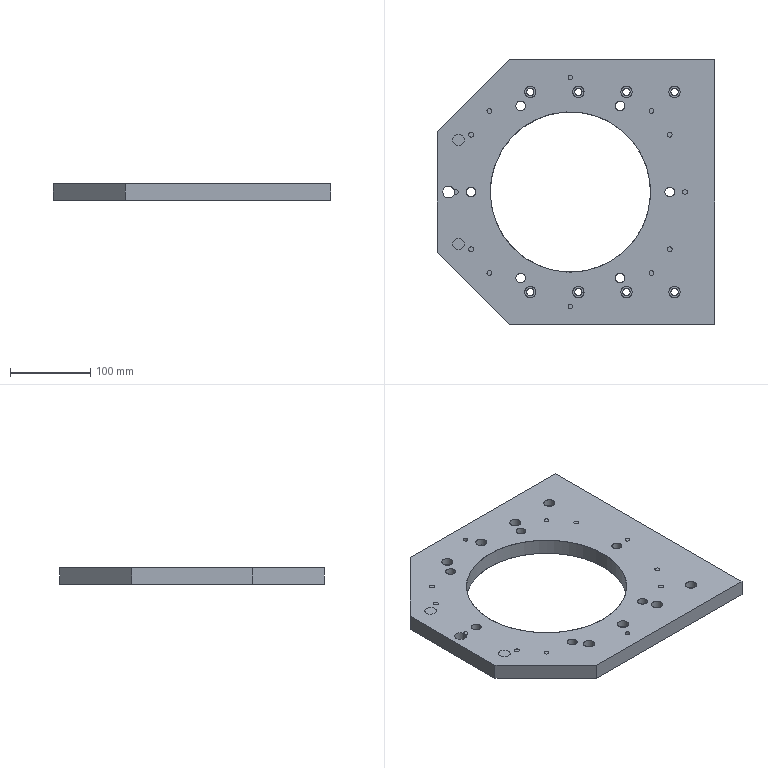NC program | NX | posted with a generic post | part box 346 x 330 x 20 mm
Lines 1 to 1039 of 2811:
N10 G17 G21 G94 G90
(ZLEVEL_PROFILE_COPY_1_1 , TOOL : D10)
N12 T10 M6
N14 G54
N16 G17 G0 G90 X174.775 Y181.218 S2200 M3
N18 G43 Z70. H10
N20 Z2.78
N22 G94 G1 Z-0.22 F2200.
N24 X170.649 Y178.835
N26 G3 X170.149 Y177.969 R1.
N28 G1 X170.15 Y173.041
N30 Y-83.
N32 G2 X168.642 Y-86.642 R5.15
N34 G1 X78.642 Y-176.642
N36 X74.993 Y-180.29
N38 G3 X74.734 Y-181.256 R1.
N40 G1 X75.955 Y-185.815
N42 Z2.78
N44 G0 Z2.56
N46 G1 Z-0.44
N48 X74.734 Y-181.256
N50 G2 X74.993 Y-180.29 R1.
N52 G1 X78.642 Y-176.642
N54 X168.642 Y-86.642
N56 G3 X170.15 Y-83. R5.15
N58 G1 Y173.041
N60 X170.149 Y177.969
N62 G2 X170.649 Y178.835 R1.
N64 G1 X174.775 Y181.218
N66 Z2.56
N68 G0 Z2.341
N70 G1 Z-0.659
N72 X170.649 Y178.835
N74 G3 X170.149 Y177.969 R1.
N76 G1 X170.15 Y173.041
N78 Y-83.
N80 G2 X168.642 Y-86.642 R5.15
N82 G1 X78.642 Y-176.642
N84 X74.993 Y-180.29
N86 G3 X74.734 Y-181.256 R1.
N88 G1 X75.955 Y-185.815
N90 Z2.341
N92 G0 Z2.121
N94 G1 Z-0.879
N96 X74.734 Y-181.256
N98 G2 X74.993 Y-180.29 R1.
N100 G1 X78.642 Y-176.642
N102 X168.642 Y-86.642
N104 G3 X170.15 Y-83. R5.15
N106 G1 Y173.041
N108 X170.149 Y177.969
N110 G2 X170.649 Y178.835 R1.
N112 G1 X174.775 Y181.218
N114 Z2.121
N116 G0 Z1.901
N118 G1 Z-1.099
N120 X170.649 Y178.835
N122 G3 X170.149 Y177.969 R1.
N124 G1 X170.15 Y173.041
N126 Y-83.
N128 G2 X168.642 Y-86.642 R5.15
N130 G1 X78.642 Y-176.642
N132 X74.993 Y-180.29
N134 G3 X74.734 Y-181.256 R1.
N136 G1 X75.955 Y-185.815
N138 Z1.901
N140 G0 Z1.681
N142 G1 Z-1.319
N144 X74.734 Y-181.256
N146 G2 X74.993 Y-180.29 R1.
N148 G1 X78.642 Y-176.642
N150 X168.642 Y-86.642
N152 G3 X170.15 Y-83. R5.15
N154 G1 Y173.041
N156 X170.149 Y177.969
N158 G2 X170.649 Y178.835 R1.
N160 G1 X174.775 Y181.218
N162 Z1.681
N164 G0 Z1.462
N166 G1 Z-1.538
N168 X170.649 Y178.835
N170 G3 X170.149 Y177.969 R1.
N172 G1 X170.15 Y173.041
N174 Y-83.
N176 G2 X168.642 Y-86.642 R5.15
N178 G1 X78.642 Y-176.642
N180 X74.993 Y-180.29
N182 G3 X74.734 Y-181.256 R1.
N184 G1 X75.955 Y-185.815
N186 Z1.462
N188 G0 Z1.242
N190 G1 Z-1.758
N192 X74.734 Y-181.256
N194 G2 X74.993 Y-180.29 R1.
N196 G1 X78.642 Y-176.642
N198 X168.642 Y-86.642
N200 G3 X170.15 Y-83. R5.15
N202 G1 Y173.041
N204 X170.149 Y177.969
N206 G2 X170.649 Y178.835 R1.
N208 G1 X174.775 Y181.218
N210 Z1.242
N212 G0 Z1.022
N214 G1 Z-1.978
N216 X170.649 Y178.835
N218 G3 X170.149 Y177.969 R1.
N220 G1 X170.15 Y173.041
N222 Y-83.
N224 G2 X168.642 Y-86.642 R5.15
N226 G1 X78.642 Y-176.642
N228 X74.993 Y-180.29
N230 G3 X74.734 Y-181.256 R1.
N232 G1 X75.955 Y-185.815
N234 Z1.022
N236 G0 Z0.802
N238 G1 Z-2.198
N240 X74.734 Y-181.256
N242 G2 X74.993 Y-180.29 R1.
N244 G1 X78.642 Y-176.642
N246 X168.642 Y-86.642
N248 G3 X170.15 Y-83. R5.15
N250 G1 Y173.041
N252 X170.149 Y177.969
N254 G2 X170.649 Y178.835 R1.
N256 G1 X174.775 Y181.218
N258 Z0.802
N260 G0 Z0.582
N262 G1 Z-2.418
N264 X170.649 Y178.835
N266 G3 X170.149 Y177.969 R1.
N268 G1 X170.15 Y173.041
N270 Y-83.
N272 G2 X168.642 Y-86.642 R5.15
N274 G1 X78.642 Y-176.642
N276 X74.993 Y-180.29
N278 G3 X74.734 Y-181.256 R1.
N280 G1 X75.955 Y-185.815
N282 Z0.582
N284 G0 Z0.363
N286 G1 Z-2.637
N288 X74.734 Y-181.256
N290 G2 X74.993 Y-180.29 R1.
N292 G1 X78.642 Y-176.642
N294 X168.642 Y-86.642
N296 G3 X170.15 Y-83. R5.15
N298 G1 Y173.041
N300 X170.149 Y177.969
N302 G2 X170.649 Y178.835 R1.
N304 G1 X174.775 Y181.218
N306 Z0.363
N308 G0 Z0.143
N310 G1 Z-2.857
N312 X170.649 Y178.835
N314 G3 X170.149 Y177.969 R1.
N316 G1 X170.15 Y173.041
N318 Y-83.
N320 G2 X168.642 Y-86.642 R5.15
N322 G1 X78.642 Y-176.642
N324 X74.993 Y-180.29
N326 G3 X74.734 Y-181.256 R1.
N328 G1 X75.955 Y-185.815
N330 Z0.143
N332 G0 Z-0.077
N334 G1 Z-3.077
N336 X74.734 Y-181.256
N338 G2 X74.993 Y-180.29 R1.
N340 G1 X78.642 Y-176.642
N342 X168.642 Y-86.642
N344 G3 X170.15 Y-83. R5.15
N346 G1 Y173.041
N348 X170.149 Y177.969
N350 G2 X170.649 Y178.835 R1.
N352 G1 X174.775 Y181.218
N354 Z-0.077
N356 G0 Z-0.297
N358 G1 Z-3.297
N360 X170.649 Y178.835
N362 G3 X170.149 Y177.969 R1.
N364 G1 X170.15 Y173.041
N366 Y-83.
N368 G2 X168.642 Y-86.642 R5.15
N370 G1 X78.642 Y-176.642
N372 X74.993 Y-180.29
N374 G3 X74.734 Y-181.256 R1.
N376 G1 X75.955 Y-185.815
N378 Z-0.297
N380 G0 Z-0.516
N382 G1 Z-3.516
N384 X74.734 Y-181.256
N386 G2 X74.993 Y-180.29 R1.
N388 G1 X78.642 Y-176.642
N390 X168.642 Y-86.642
N392 G3 X170.15 Y-83. R5.15
N394 G1 Y173.041
N396 X170.149 Y177.969
N398 G2 X170.649 Y178.835 R1.
N400 G1 X174.775 Y181.218
N402 Z-0.516
N404 G0 Z-0.736
N406 G1 Z-3.736
N408 X170.649 Y178.835
N410 G3 X170.149 Y177.969 R1.
N412 G1 X170.15 Y173.041
N414 Y-83.
N416 G2 X168.642 Y-86.642 R5.15
N418 G1 X78.642 Y-176.642
N420 X74.993 Y-180.29
N422 G3 X74.734 Y-181.256 R1.
N424 G1 X75.955 Y-185.815
N426 Z-0.736
N428 G0 Z-0.956
N430 G1 Z-3.956
N432 X74.734 Y-181.256
N434 G2 X74.993 Y-180.29 R1.
N436 G1 X78.642 Y-176.642
N438 X168.642 Y-86.642
N440 G3 X170.15 Y-83. R5.15
N442 G1 Y173.041
N444 X170.149 Y177.969
N446 G2 X170.649 Y178.835 R1.
N448 G1 X174.775 Y181.218
N450 Z-0.956
N452 G0 Z-1.176
N454 G1 Z-4.176
N456 X170.649 Y178.835
N458 G3 X170.149 Y177.969 R1.
N460 G1 X170.15 Y173.041
N462 Y-83.
N464 G2 X168.642 Y-86.642 R5.15
N466 G1 X78.642 Y-176.642
N468 X74.993 Y-180.29
N470 G3 X74.734 Y-181.256 R1.
N472 G1 X75.955 Y-185.815
N474 Z-1.176
N476 G0 Z-1.396
N478 G1 Z-4.396
N480 X74.734 Y-181.256
N482 G2 X74.993 Y-180.29 R1.
N484 G1 X78.642 Y-176.642
N486 X168.642 Y-86.642
N488 G3 X170.15 Y-83. R5.15
N490 G1 Y173.041
N492 X170.149 Y177.969
N494 G2 X170.649 Y178.835 R1.
N496 G1 X174.775 Y181.218
N498 Z-1.396
N500 G0 Z-1.615
N502 G1 Z-4.615
N504 X170.649 Y178.835
N506 G3 X170.149 Y177.969 R1.
N508 G1 X170.15 Y173.041
N510 Y-83.
N512 G2 X168.642 Y-86.642 R5.15
N514 G1 X78.642 Y-176.642
N516 X74.993 Y-180.29
N518 G3 X74.734 Y-181.256 R1.
N520 G1 X75.955 Y-185.815
N522 Z-1.615
N524 G0 Z-1.835
N526 G1 Z-4.835
N528 X74.734 Y-181.256
N530 G2 X74.993 Y-180.29 R1.
N532 G1 X78.642 Y-176.642
N534 X168.642 Y-86.642
N536 G3 X170.15 Y-83. R5.15
N538 G1 Y173.041
N540 X170.149 Y177.969
N542 G2 X170.649 Y178.835 R1.
N544 G1 X174.775 Y181.218
N546 Z-1.835
N548 G0 Z-2.055
N550 G1 Z-5.055
N552 X170.649 Y178.835
N554 G3 X170.149 Y177.969 R1.
N556 G1 X170.15 Y173.041
N558 Y-83.
N560 G2 X168.642 Y-86.642 R5.15
N562 G1 X78.642 Y-176.642
N564 X74.993 Y-180.29
N566 G3 X74.734 Y-181.256 R1.
N568 G1 X75.955 Y-185.815
N570 Z-2.055
N572 G0 Z-2.275
N574 G1 Z-5.275
N576 X74.734 Y-181.256
N578 G2 X74.993 Y-180.29 R1.
N580 G1 X78.642 Y-176.642
N582 X168.642 Y-86.642
N584 G3 X170.15 Y-83. R5.15
N586 G1 Y173.041
N588 X170.149 Y177.969
N590 G2 X170.649 Y178.835 R1.
N592 G1 X174.775 Y181.218
N594 Z-2.275
N596 G0 Z-2.495
N598 G1 Z-5.495
N600 X170.649 Y178.835
N602 G3 X170.149 Y177.969 R1.
N604 G1 X170.15 Y173.041
N606 Y-83.
N608 G2 X168.642 Y-86.642 R5.15
N610 G1 X78.642 Y-176.642
N612 X74.993 Y-180.29
N614 G3 X74.734 Y-181.256 R1.
N616 G1 X75.955 Y-185.815
N618 Z-2.495
N620 G0 Z-2.714
N622 G1 Z-5.714
N624 X74.734 Y-181.256
N626 G2 X74.993 Y-180.29 R1.
N628 G1 X78.642 Y-176.642
N630 X168.642 Y-86.642
N632 G3 X170.15 Y-83. R5.15
N634 G1 Y173.041
N636 X170.149 Y177.969
N638 G2 X170.649 Y178.835 R1.
N640 G1 X174.775 Y181.218
N642 Z-2.714
N644 G0 Z-2.934
N646 G1 Z-5.934
N648 X170.649 Y178.835
N650 G3 X170.149 Y177.969 R1.
N652 G1 X170.15 Y173.041
N654 Y-83.
N656 G2 X168.642 Y-86.642 R5.15
N658 G1 X78.642 Y-176.642
N660 X74.993 Y-180.29
N662 G3 X74.734 Y-181.256 R1.
N664 G1 X75.955 Y-185.815
N666 Z-2.934
N668 G0 Z-3.154
N670 G1 Z-6.154
N672 X74.734 Y-181.256
N674 G2 X74.993 Y-180.29 R1.
N676 G1 X78.642 Y-176.642
N678 X168.642 Y-86.642
N680 G3 X170.15 Y-83. R5.15
N682 G1 Y173.041
N684 X170.149 Y177.969
N686 G2 X170.649 Y178.835 R1.
N688 G1 X174.775 Y181.218
N690 Z-3.154
N692 G0 Z-3.374
N694 G1 Z-6.374
N696 X170.649 Y178.835
N698 G3 X170.149 Y177.969 R1.
N700 G1 X170.15 Y173.041
N702 Y-83.
N704 G2 X168.642 Y-86.642 R5.15
N706 G1 X78.642 Y-176.642
N708 X74.993 Y-180.29
N710 G3 X74.734 Y-181.256 R1.
N712 G1 X75.955 Y-185.815
N714 Z-3.374
N716 G0 Z-3.593
N718 G1 Z-6.593
N720 X74.734 Y-181.256
N722 G2 X74.993 Y-180.29 R1.
N724 G1 X78.642 Y-176.642
N726 X168.642 Y-86.642
N728 G3 X170.15 Y-83. R5.15
N730 G1 Y173.041
N732 X170.149 Y177.969
N734 G2 X170.649 Y178.835 R1.
N736 G1 X174.775 Y181.218
N738 Z-3.593
N740 G0 Z-3.813
N742 G1 Z-6.813
N744 X170.649 Y178.835
N746 G3 X170.149 Y177.969 R1.
N748 G1 X170.15 Y173.041
N750 Y-83.
N752 G2 X168.642 Y-86.642 R5.15
N754 G1 X78.642 Y-176.642
N756 X74.993 Y-180.29
N758 G3 X74.734 Y-181.256 R1.
N760 G1 X75.955 Y-185.815
N762 Z-3.813
N764 G0 Z-4.033
N766 G1 Z-7.033
N768 X74.734 Y-181.256
N770 G2 X74.993 Y-180.29 R1.
N772 G1 X78.642 Y-176.642
N774 X168.642 Y-86.642
N776 G3 X170.15 Y-83. R5.15
N778 G1 Y173.041
N780 X170.149 Y177.969
N782 G2 X170.649 Y178.835 R1.
N784 G1 X174.775 Y181.218
N786 Z-4.033
N788 G0 Z-4.253
N790 G1 Z-7.253
N792 X170.649 Y178.835
N794 G3 X170.149 Y177.969 R1.
N796 G1 X170.15 Y173.041
N798 Y-83.
N800 G2 X168.642 Y-86.642 R5.15
N802 G1 X78.642 Y-176.642
N804 X74.993 Y-180.29
N806 G3 X74.734 Y-181.256 R1.
N808 G1 X75.955 Y-185.815
N810 Z-4.253
N812 G0 Z-4.473
N814 G1 Z-7.473
N816 X74.734 Y-181.256
N818 G2 X74.993 Y-180.29 R1.
N820 G1 X78.642 Y-176.642
N822 X168.642 Y-86.642
N824 G3 X170.15 Y-83. R5.15
N826 G1 Y173.041
N828 X170.149 Y177.969
N830 G2 X170.649 Y178.835 R1.
N832 G1 X174.775 Y181.218
N834 Z-4.473
N836 G0 Z-4.692
N838 G1 Z-7.692
N840 X170.649 Y178.835
N842 G3 X170.149 Y177.969 R1.
N844 G1 X170.15 Y173.041
N846 Y-83.
N848 G2 X168.642 Y-86.642 R5.15
N850 G1 X78.642 Y-176.642
N852 X74.993 Y-180.29
N854 G3 X74.734 Y-181.256 R1.
N856 G1 X75.955 Y-185.815
N858 Z-4.692
N860 G0 Z-4.912
N862 G1 Z-7.912
N864 X74.734 Y-181.256
N866 G2 X74.993 Y-180.29 R1.
N868 G1 X78.642 Y-176.642
N870 X168.642 Y-86.642
N872 G3 X170.15 Y-83. R5.15
N874 G1 Y173.041
N876 X170.149 Y177.969
N878 G2 X170.649 Y178.835 R1.
N880 G1 X174.775 Y181.218
N882 Z-4.912
N884 G0 Z-5.132
N886 G1 Z-8.132
N888 X170.649 Y178.835
N890 G3 X170.149 Y177.969 R1.
N892 G1 X170.15 Y173.041
N894 Y-83.
N896 G2 X168.642 Y-86.642 R5.15
N898 G1 X78.642 Y-176.642
N900 X74.993 Y-180.29
N902 G3 X74.734 Y-181.256 R1.
N904 G1 X75.955 Y-185.815
N906 Z-5.132
N908 G0 Z-5.352
N910 G1 Z-8.352
N912 X74.734 Y-181.256
N914 G2 X74.993 Y-180.29 R1.
N916 G1 X78.642 Y-176.642
N918 X168.642 Y-86.642
N920 G3 X170.15 Y-83. R5.15
N922 G1 Y173.041
N924 X170.149 Y177.969
N926 G2 X170.649 Y178.835 R1.
N928 G1 X174.775 Y181.218
N930 Z-5.352
N932 G0 Z-5.571
N934 G1 Z-8.571
N936 X170.649 Y178.835
N938 G3 X170.149 Y177.969 R1.
N940 G1 X170.15 Y173.041
N942 Y-83.
N944 G2 X168.642 Y-86.642 R5.15
N946 G1 X78.642 Y-176.642
N948 X74.993 Y-180.29
N950 G3 X74.734 Y-181.256 R1.
N952 G1 X75.955 Y-185.815
N954 Z-5.571
N956 G0 Z-5.791
N958 G1 Z-8.791
N960 X74.734 Y-181.256
N962 G2 X74.993 Y-180.29 R1.
N964 G1 X78.642 Y-176.642
N966 X168.642 Y-86.642
N968 G3 X170.15 Y-83. R5.15
N970 G1 Y173.041
N972 X170.149 Y177.969
N974 G2 X170.649 Y178.835 R1.
N976 G1 X174.775 Y181.218
N978 Z-5.791
N980 G0 Z-6.011
N982 G1 Z-9.011
N984 X170.649 Y178.835
N986 G3 X170.149 Y177.969 R1.
N988 G1 X170.15 Y173.041
N990 Y-83.
N992 G2 X168.642 Y-86.642 R5.15
N994 G1 X78.642 Y-176.642
N996 X74.993 Y-180.29
N998 G3 X74.734 Y-181.256 R1.
N1000 G1 X75.955 Y-185.815
N1002 Z-6.011
N1004 G0 Z-6.231
N1006 G1 Z-9.231
N1008 X74.734 Y-181.256
N1010 G2 X74.993 Y-180.29 R1.
N1012 G1 X78.642 Y-176.642
N1014 X168.642 Y-86.642
N1016 G3 X170.15 Y-83. R5.15
N1018 G1 Y173.041
N1020 X170.149 Y177.969
N1022 G2 X170.649 Y178.835 R1.
N1024 G1 X174.775 Y181.218
N1026 Z-6.231
N1028 G0 Z-6.451
N1030 G1 Z-9.451
N1032 X170.649 Y178.835
N1034 G3 X170.149 Y177.969 R1.
N1036 G1 X170.15 Y173.041
N1038 Y-83.
N1040 G2 X168.642 Y-86.642 R5.15
N1042 G1 X78.642 Y-176.642
N1044 X74.993 Y-180.29
N1046 G3 X74.734 Y-181.256 R1.
N1048 G1 X75.955 Y-185.815
N1050 Z-6.451
N1052 G0 Z-6.67
N1054 G1 Z-9.67
N1056 X74.734 Y-181.256
N1058 G2 X74.993 Y-180.29 R1.
N1060 G1 X78.642 Y-176.642
N1062 X168.642 Y-86.642
N1064 G3 X170.15 Y-83. R5.15
N1066 G1 Y173.041
N1068 X170.149 Y177.969
N1070 G2 X170.649 Y178.835 R1.
N1072 G1 X174.775 Y181.218
N1074 Z-6.67
N1076 G0 Z-6.89
N1078 G1 Z-9.89
N1080 X170.649 Y178.835
N1082 G3 X170.149 Y177.969 R1.
N1084 G1 X170.15 Y173.041
N1086 Y-83.
N1088 G2 X168.642 Y-86.642 R5.15
N1090 G1 X78.642 Y-176.642
N1092 X74.993 Y-180.29
N1094 G3 X74.734 Y-181.256 R1.
N1096 G1 X75.955 Y-185.815
N1098 Z-6.89
N1100 G0 Z-7.11
N1102 G1 Z-10.11
N1104 X74.734 Y-181.256
N1106 G2 X74.993 Y-180.29 R1.
N1108 G1 X78.642 Y-176.642
N1110 X168.642 Y-86.642
N1112 G3 X170.15 Y-83. R5.15
N1114 G1 Y173.041
N1116 X170.149 Y177.969
N1118 G2 X170.649 Y178.835 R1.
N1120 G1 X174.775 Y181.218
N1122 Z-7.11
N1124 G0 Z-7.33
N1126 G1 Z-10.33
N1128 X170.649 Y178.835
N1130 G3 X170.149 Y177.969 R1.
N1132 G1 X170.15 Y173.041
N1134 Y-83.
N1136 G2 X168.642 Y-86.642 R5.15
N1138 G1 X78.642 Y-176.642
N1140 X74.993 Y-180.29
N1142 G3 X74.734 Y-181.256 R1.
N1144 G1 X75.955 Y-185.815
N1146 Z-7.33
N1148 G0 Z-7.549
N1150 G1 Z-10.549
N1152 X74.734 Y-181.256
N1154 G2 X74.993 Y-180.29 R1.
N1156 G1 X78.642 Y-176.642
N1158 X168.642 Y-86.642
N1160 G3 X170.15 Y-83. R5.15
N1162 G1 Y173.041
N1164 X170.149 Y177.969
N1166 G2 X170.649 Y178.835 R1.
N1168 G1 X174.775 Y181.218
N1170 Z-7.549
N1172 G0 Y181.217 Z-7.769
N1174 G1 Z-10.769
N1176 X170.649 Y178.835
N1178 G3 X170.149 Y177.969 R1.
N1180 G1 X170.15 Y173.041
N1182 Y-83.
N1184 G2 X168.642 Y-86.642 R5.15
N1186 G1 X78.642 Y-176.642
N1188 X74.993 Y-180.29
N1190 G3 X74.734 Y-181.256 R1.
N1192 G1 X75.955 Y-185.816
N1194 Z-7.769
N1196 G0 Z-7.989
N1198 G1 Z-10.989
N1200 X74.734 Y-181.256
N1202 G2 X74.993 Y-180.29 R1.
N1204 G1 X78.642 Y-176.642
N1206 X168.642 Y-86.642
N1208 G3 X170.15 Y-83. R5.15
N1210 G1 Y173.041
N1212 X170.149 Y177.969
N1214 G2 X170.649 Y178.835 R1.
N1216 G1 X174.775 Y181.217
N1218 Z-7.989
N1220 G0 Z-8.209
N1222 G1 Z-11.209
N1224 X170.649 Y178.835
N1226 G3 X170.149 Y177.969 R1.
N1228 G1 X170.15 Y173.041
N1230 Y-83.
N1232 G2 X168.642 Y-86.642 R5.15
N1234 G1 X78.642 Y-176.642
N1236 X74.993 Y-180.29
N1238 G3 X74.734 Y-181.256 R1.
N1240 G1 X75.955 Y-185.816
N1242 Z-8.209
N1244 G0 Z-8.429
N1246 G1 Z-11.429
N1248 X74.734 Y-181.256
N1250 G2 X74.993 Y-180.29 R1.
N1252 G1 X78.642 Y-176.642
N1254 X168.642 Y-86.642
N1256 G3 X170.15 Y-83. R5.15
N1258 G1 Y173.041
N1260 X170.149 Y177.969
N1262 G2 X170.649 Y178.835 R1.
N1264 G1 X174.775 Y181.217
N1266 Z-8.429
N1268 G0 Z-8.648
N1270 G1 Z-11.648
N1272 X170.649 Y178.835
N1274 G3 X170.149 Y177.969 R1.
N1276 G1 X170.15 Y173.041
N1278 Y-83.
N1280 G2 X168.642 Y-86.642 R5.15
N1282 G1 X78.642 Y-176.642
N1284 X74.993 Y-180.29
N1286 G3 X74.734 Y-181.256 R1.
N1288 G1 X75.955 Y-185.816
N1290 Z-8.648
N1292 G0 Z-8.868
N1294 G1 Z-11.868
N1296 X74.734 Y-181.256
N1298 G2 X74.993 Y-180.29 R1.
N1300 G1 X78.642 Y-176.642
N1302 X168.642 Y-86.642
N1304 G3 X170.15 Y-83. R5.15
N1306 G1 Y173.041
N1308 X170.149 Y177.969
N1310 G2 X170.649 Y178.835 R1.
N1312 G1 X174.775 Y181.217
N1314 Z-8.868
N1316 G0 Z-9.088
N1318 G1 Z-12.088
N1320 X170.649 Y178.835
N1322 G3 X170.149 Y177.969 R1.
N1324 G1 X170.15 Y173.041
N1326 Y-83.
N1328 G2 X168.642 Y-86.642 R5.15
N1330 G1 X78.642 Y-176.642
N1332 X74.993 Y-180.29
N1334 G3 X74.734 Y-181.256 R1.
N1336 G1 X75.955 Y-185.816
N1338 Z-9.088
N1340 G0 Z-9.308
N1342 G1 Z-12.308
N1344 X74.734 Y-181.256
N1346 G2 X74.993 Y-180.29 R1.
N1348 G1 X78.642 Y-176.642
N1350 X168.642 Y-86.642
N1352 G3 X170.15 Y-83. R5.15
N1354 G1 Y173.041
N1356 X170.149 Y177.969
N1358 G2 X170.649 Y178.835 R1.
N1360 G1 X174.775 Y181.217
N1362 Z-9.308
N1364 G0 Z-9.527
N1366 G1 Z-12.527
N1368 X170.649 Y178.835
N1370 G3 X170.149 Y177.969 R1.
N1372 G1 X170.15 Y173.041
N1374 Y-83.
N1376 G2 X168.642 Y-86.642 R5.15
N1378 G1 X78.642 Y-176.642
N1380 X74.993 Y-180.29
N1382 G3 X74.734 Y-181.256 R1.
N1384 G1 X75.955 Y-185.816
N1386 Z-9.527
N1388 G0 Z-9.747
N1390 G1 Z-12.747
N1392 X74.734 Y-181.256
N1394 G2 X74.993 Y-180.29 R1.
N1396 G1 X78.642 Y-176.642
N1398 X168.642 Y-86.642
N1400 G3 X170.15 Y-83. R5.15
N1402 G1 Y173.041
N1404 X170.149 Y177.969
N1406 G2 X170.649 Y178.835 R1.
N1408 G1 X174.775 Y181.217
N1410 Z-9.747
N1412 G0 Z-9.967
N1414 G1 Z-12.967
N1416 X170.649 Y178.835
N1418 G3 X170.149 Y177.969 R1.
N1420 G1 X170.15 Y173.041
N1422 Y-83.
N1424 G2 X168.642 Y-86.642 R5.15
N1426 G1 X78.642 Y-176.642
N1428 X74.993 Y-180.29
N1430 G3 X74.734 Y-181.256 R1.
N1432 G1 X75.955 Y-185.816
N1434 Z-9.967
N1436 G0 Z-10.187
N1438 G1 Z-13.187
N1440 X74.734 Y-181.256
N1442 G2 X74.993 Y-180.29 R1.
N1444 G1 X78.642 Y-176.642
N1446 X168.642 Y-86.642
N1448 G3 X170.15 Y-83. R5.15
N1450 G1 Y173.041
N1452 X170.149 Y177.969
N1454 G2 X170.649 Y178.835 R1.
N1456 G1 X174.775 Y181.217
N1458 Z-10.187
N1460 G0 Z-10.407
N1462 G1 Z-13.407
N1464 X170.649 Y178.835
N1466 G3 X170.149 Y177.969 R1.
N1468 G1 X170.15 Y173.041
N1470 Y-83.
N1472 G2 X168.642 Y-86.642 R5.15
N1474 G1 X78.642 Y-176.642
N1476 X74.993 Y-180.29
N1478 G3 X74.734 Y-181.256 R1.
N1480 G1 X75.955 Y-185.816
N1482 Z-10.407
N1484 G0 Z-10.626
N1486 G1 Z-13.626
N1488 X74.734 Y-181.256
N1490 G2 X74.993 Y-180.29 R1.
N1492 G1 X78.642 Y-176.642
N1494 X168.642 Y-86.642
N1496 G3 X170.15 Y-83. R5.15
N1498 G1 Y173.041
N1500 X170.149 Y177.969
N1502 G2 X170.649 Y178.835 R1.
N1504 G1 X174.775 Y181.217
N1506 Z-10.626
N1508 G0 Z-10.846
N1510 G1 Z-13.846
N1512 X170.649 Y178.835
N1514 G3 X170.149 Y177.969 R1.
N1516 G1 X170.15 Y173.041
N1518 Y-83.
N1520 G2 X168.642 Y-86.642 R5.15
N1522 G1 X78.642 Y-176.642
N1524 X74.993 Y-180.29
N1526 G3 X74.734 Y-181.256 R1.
N1528 G1 X75.955 Y-185.816
N1530 Z-10.846
N1532 G0 Z-11.066
N1534 G1 Z-14.066
N1536 X74.734 Y-181.256
N1538 G2 X74.993 Y-180.29 R1.
N1540 G1 X78.642 Y-176.642
N1542 X168.642 Y-86.642
N1544 G3 X170.15 Y-83. R5.15
N1546 G1 Y173.041
N1548 X170.149 Y177.969
N1550 G2 X170.649 Y178.835 R1.
N1552 G1 X174.775 Y181.217
N1554 Z-11.066
N1556 G0 Z-11.286
N1558 G1 Z-14.286
N1560 X170.649 Y178.835
N1562 G3 X170.149 Y177.969 R1.
N1564 G1 X170.15 Y173.041
N1566 Y-83.
N1568 G2 X168.642 Y-86.642 R5.15
N1570 G1 X78.642 Y-176.642
N1572 X74.993 Y-180.29
N1574 G3 X74.734 Y-181.256 R1.
N1576 G1 X75.955 Y-185.816
N1578 Z-11.286
N1580 G0 X75.956 Z-11.505
N1582 G1 Z-14.505
N1584 X74.734 Y-181.256
N1586 G2 X74.993 Y-180.29 R1.
N1588 G1 X78.642 Y-176.642
N1590 X168.642 Y-86.642
N1592 G3 X170.15 Y-83. R5.15
N1594 G1 Y173.041
N1596 X170.149 Y177.969
N1598 G2 X170.649 Y178.835 R1.
N1600 G1 X174.775 Y181.217
N1602 Z-11.505
N1604 G0 Z-11.725
N1606 G1 Z-14.725
N1608 X170.649 Y178.835
N1610 G3 X170.149 Y177.969 R1.
N1612 G1 X170.15 Y173.041
N1614 Y-83.
N1616 G2 X168.642 Y-86.642 R5.15
N1618 G1 X78.642 Y-176.642
N1620 X74.993 Y-180.29
N1622 G3 X74.734 Y-181.256 R1.
N1624 G1 X75.956 Y-185.816
N1626 Z-11.725
N1628 G0 Z-11.945
N1630 G1 Z-14.945
N1632 X74.734 Y-181.256
N1634 G2 X74.993 Y-180.29 R1.
N1636 G1 X78.642 Y-176.642
N1638 X168.642 Y-86.642
N1640 G3 X170.15 Y-83. R5.15
N1642 G1 Y173.041
N1644 X170.149 Y177.969
N1646 G2 X170.649 Y178.835 R1.
N1648 G1 X174.775 Y181.217
N1650 Z-11.945
N1652 G0 Z-12.165
N1654 G1 Z-15.165
N1656 X170.649 Y178.835
N1658 G3 X170.149 Y177.969 R1.
N1660 G1 X170.15 Y173.041
N1662 Y-83.
N1664 G2 X168.642 Y-86.642 R5.15
N1666 G1 X78.642 Y-176.642
N1668 X74.993 Y-180.29
N1670 G3 X74.734 Y-181.256 R1.
N1672 G1 X75.956 Y-185.816
N1674 Z-12.165
N1676 G0 Z-12.385
N1678 G1 Z-15.385
N1680 X74.734 Y-181.256
N1682 G2 X74.993 Y-180.29 R1.
N1684 G1 X78.642 Y-176.642
N1686 X168.642 Y-86.642
N1688 G3 X170.15 Y-83. R5.15
N1690 G1 Y173.041
N1692 X170.149 Y177.969
N1694 G2 X170.649 Y178.835 R1.
N1696 G1 X174.775 Y181.217
N1698 Z-12.385
N1700 G0 Z-12.604
N1702 G1 Z-15.604
N1704 X170.649 Y178.835
N1706 G3 X170.149 Y177.969 R1.
N1708 G1 X170.15 Y173.041
N1710 Y-83.
N1712 G2 X168.642 Y-86.642 R5.15
N1714 G1 X78.642 Y-176.642
N1716 X74.993 Y-180.29
N1718 G3 X74.734 Y-181.256 R1.
N1720 G1 X75.956 Y-185.816
N1722 Z-12.604
N1724 G0 Z-12.824
N1726 G1 Z-15.824
N1728 X74.734 Y-181.256
N1730 G2 X74.993 Y-180.29 R1.
N1732 G1 X78.642 Y-176.642
N1734 X168.642 Y-86.642
N1736 G3 X170.15 Y-83. R5.15
N1738 G1 Y173.041
N1740 X170.149 Y177.969
N1742 G2 X170.649 Y178.835 R1.
N1744 G1 X174.775 Y181.217
N1746 Z-12.824
N1748 G0 Z-13.044
N1750 G1 Z-16.044
N1752 X170.649 Y178.835
N1754 G3 X170.149 Y177.969 R1.
N1756 G1 X170.15 Y173.041
N1758 Y-83.
N1760 G2 X168.642 Y-86.642 R5.15
N1762 G1 X78.642 Y-176.642
N1764 X74.993 Y-180.29
N1766 G3 X74.734 Y-181.256 R1.
N1768 G1 X75.956 Y-185.816
N1770 Z-13.044
N1772 G0 Z-13.264
N1774 G1 Z-16.264
N1776 X74.734 Y-181.256
N1778 G2 X74.993 Y-180.29 R1.
N1780 G1 X78.642 Y-176.642
N1782 X168.642 Y-86.642
N1784 G3 X170.15 Y-83. R5.15
N1786 G1 Y173.041
N1788 X170.149 Y177.969
N1790 G2 X170.649 Y178.835 R1.
N1792 G1 X174.775 Y181.217
N1794 Z-13.264
N1796 G0 Z-13.484
N1798 G1 Z-16.484
N1800 X170.649 Y178.835
N1802 G3 X170.149 Y177.969 R1.
N1804 G1 X170.15 Y173.041
N1806 Y-83.
N1808 G2 X168.642 Y-86.642 R5.15
N1810 G1 X78.642 Y-176.642
N1812 X74.993 Y-180.29
N1814 G3 X74.734 Y-181.256 R1.
N1816 G1 X75.956 Y-185.816
N1818 Z-13.484
N1820 G0 Z-13.703
N1822 G1 Z-16.703
N1824 X74.734 Y-181.256
N1826 G2 X74.993 Y-180.29 R1.
N1828 G1 X78.642 Y-176.642
N1830 X168.642 Y-86.642
N1832 G3 X170.15 Y-83. R5.15
N1834 G1 Y173.041
N1836 X170.149 Y177.969
N1838 G2 X170.649 Y178.835 R1.
N1840 G1 X174.775 Y181.217
N1842 Z-13.703
N1844 G0 Z-13.923
N1846 G1 Z-16.923
N1848 X170.649 Y178.835
N1850 G3 X170.149 Y177.969 R1.
N1852 G1 X170.15 Y173.041
N1854 Y-83.
N1856 G2 X168.642 Y-86.642 R5.15
N1858 G1 X78.642 Y-176.642
N1860 X74.993 Y-180.29
N1862 G3 X74.734 Y-181.256 R1.
N1864 G1 X75.956 Y-185.816
N1866 Z-13.923
N1868 G0 Z-14.143
N1870 G1 Z-17.143
N1872 X74.734 Y-181.256
N1874 G2 X74.993 Y-180.29 R1.
N1876 G1 X78.642 Y-176.642
N1878 X168.642 Y-86.642
N1880 G3 X170.15 Y-83. R5.15
N1882 G1 Y173.041
N1884 X170.149 Y177.969
N1886 G2 X170.649 Y178.835 R1.
N1888 G1 X174.775 Y181.217
N1890 Z-14.143
N1892 G0 Z-14.363
N1894 G1 Z-17.363
N1896 X170.649 Y178.835
N1898 G3 X170.149 Y177.969 R1.
N1900 G1 X170.15 Y173.041
N1902 Y-83.
N1904 G2 X168.642 Y-86.642 R5.15
N1906 G1 X78.642 Y-176.642
N1908 X74.993 Y-180.29
N1910 G3 X74.734 Y-181.256 R1.
N1912 G1 X75.956 Y-185.816
N1914 Z-14.363
N1916 G0 Z-14.582
N1918 G1 Z-17.582
N1920 X74.734 Y-181.256
N1922 G2 X74.993 Y-180.29 R1.
N1924 G1 X78.642 Y-176.642
N1926 X168.642 Y-86.642
N1928 G3 X170.15 Y-83. R5.15
N1930 G1 Y173.041
N1932 X170.149 Y177.969
N1934 G2 X170.649 Y178.835 R1.
N1936 G1 X174.775 Y181.217
N1938 Z-14.582
N1940 G0 Z-14.802
N1942 G1 Z-17.802
N1944 X170.649 Y178.835
N1946 G3 X170.149 Y177.969 R1.
N1948 G1 X170.15 Y173.041
N1950 Y-83.
N1952 G2 X168.642 Y-86.642 R5.15
N1954 G1 X78.642 Y-176.642
N1956 X74.993 Y-180.29
N1958 G3 X74.734 Y-181.256 R1.
N1960 G1 X75.956 Y-185.816
N1962 Z-14.802
N1964 G0 Z-15.022
N1966 G1 Z-18.022
N1968 X74.734 Y-181.256
N1970 G2 X74.993 Y-180.29 R1.
N1972 G1 X78.642 Y-176.642
N1974 X168.642 Y-86.642
N1976 G3 X170.15 Y-83. R5.15
N1978 G1 Y173.041
N1980 X170.149 Y177.969
N1982 G2 X170.649 Y178.835 R1.
N1984 G1 X174.775 Y181.217
N1986 Z-15.022
N1988 G0 Z-15.242
N1990 G1 Z-18.242
N1992 X170.649 Y178.835
N1994 G3 X170.149 Y177.969 R1.
N1996 G1 X170.15 Y173.041
N1998 Y-83.
N2000 G2 X168.642 Y-86.642 R5.15
N2002 G1 X78.642 Y-176.642
N2004 X74.993 Y-180.29
N2006 G3 X74.734 Y-181.256 R1.
N2008 G1 X75.956 Y-185.816
N2010 Z-15.242
N2012 G0 Z-15.462
N2014 G1 Z-18.462
N2016 X74.734 Y-181.256
N2018 G2 X74.993 Y-180.29 R1.
N2020 G1 X78.642 Y-176.642
N2022 X168.642 Y-86.642
N2024 G3 X170.15 Y-83. R5.15
N2026 G1 Y173.041
N2028 X170.149 Y177.969
N2030 G2 X170.649 Y178.835 R1.
N2032 G1 X174.775 Y181.217
N2034 Z-15.462
N2036 G0 Z-15.681
N2038 G1 Z-18.681
N2040 X170.649 Y178.835
N2042 G3 X170.149 Y177.969 R1.
N2044 G1 X170.15 Y173.041
N2046 Y-83.
N2048 G2 X168.642 Y-86.642 R5.15
N2050 G1 X78.642 Y-176.642
N2052 X74.993 Y-180.29
N2054 G3 X74.734 Y-181.256 R1.
N2056 G1 X75.956 Y-185.816
N2058 Z-15.681
N2060 G0 Z-15.901
N2062 G1 Z-18.901
N2064 X74.734 Y-181.256
N2066 G2 X74.993 Y-180.29 R1.
N2068 G1 X78.642 Y-176.642
N2070 X168.642 Y-86.642
N2072 G3 X170.15 Y-83. R5.15
N2074 G1 Y173.041
N2076 X170.149 Y177.969